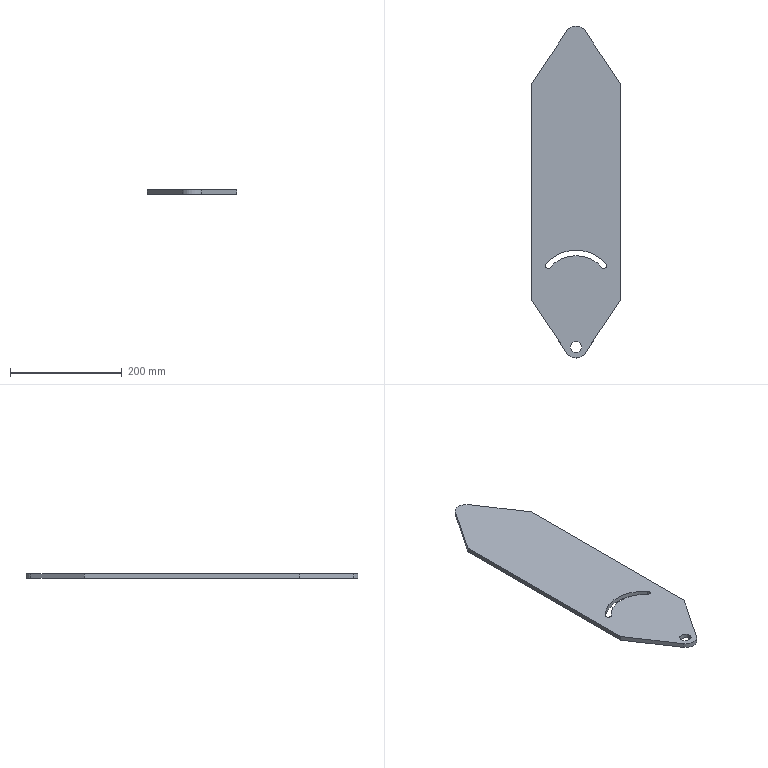Part | SolidWorks | features Cut 1, Extrusion 1 | 1 solid | 19 faces | box 160 x 594 x 8 mm | volume 632396 mm3 | plane 10 | cylinder 9 | commonest cylinder face diameters 10 x3 20 x2 40 x2 123.791 x1 143.791 x1
STEP:
#1=CARTESIAN_POINT('',(54.849,775.742,0.));
#2=VERTEX_POINT('',#1);
#3=CARTESIAN_POINT('',(53.575,779.077,0.));
#4=VERTEX_POINT('',#3);
#5=CARTESIAN_POINT('',(49.849,775.742,0.));
#6=DIRECTION('',(0.,0.,1.));
#7=DIRECTION('',(1.,0.,0.));
#8=AXIS2_PLACEMENT_3D('',#5,#6,#7);
#9=CIRCLE('',#8,5.);
#10=EDGE_CURVE('',#2,#4,#9,.T.);
#11=ORIENTED_EDGE('',*,*,#10,.F.);
#12=CARTESIAN_POINT('',(54.849,775.742,8.));
#13=VERTEX_POINT('',#12);
#14=CARTESIAN_POINT('',(54.849,775.742,-2.));
#15=DIRECTION('',(0.,0.,1.));
#16=VECTOR('',#15,1000.);
#17=LINE('',#14,#16);
#18=EDGE_CURVE('',#2,#13,#17,.T.);
#19=ORIENTED_EDGE('',*,*,#18,.T.);
#20=CARTESIAN_POINT('',(53.575,779.077,8.));
#21=VERTEX_POINT('',#20);
#22=CARTESIAN_POINT('',(49.849,775.742,8.));
#23=DIRECTION('',(0.,0.,1.));
#24=DIRECTION('',(1.,0.,0.));
#25=AXIS2_PLACEMENT_3D('',#22,#23,#24);
#26=CIRCLE('',#25,5.);
#27=EDGE_CURVE('',#13,#21,#26,.T.);
#28=ORIENTED_EDGE('',*,*,#27,.T.);
#29=CARTESIAN_POINT('',(53.575,779.077,-2.));
#30=DIRECTION('',(0.,0.,1.));
#31=VECTOR('',#30,1000.);
#32=LINE('',#29,#31);
#33=EDGE_CURVE('',#4,#21,#32,.T.);
#34=ORIENTED_EDGE('',*,*,#33,.F.);
#35=EDGE_LOOP('',(#11,#19,#28,#34));
#36=FACE_OUTER_BOUND('',#35,.T.);
#37=CARTESIAN_POINT('',(49.849,775.742,-2.));
#38=DIRECTION('',(0.,0.,1.));
#39=DIRECTION('',(1.,0.,0.));
#40=AXIS2_PLACEMENT_3D('',#37,#38,#39);
#41=CYLINDRICAL_SURFACE('',#40,5.);
#42=ADVANCED_FACE('',(#36),#41,.F.);
#43=CARTESIAN_POINT('',(-10.,630.,8.));
#44=VERTEX_POINT('',#43);
#45=CARTESIAN_POINT('',(10.,630.,8.));
#46=VERTEX_POINT('',#45);
#47=CARTESIAN_POINT('',(0.,630.,8.));
#48=DIRECTION('',(0.,0.,1.));
#49=DIRECTION('',(1.,0.,0.));
#50=AXIS2_PLACEMENT_3D('',#47,#48,#49);
#51=CIRCLE('',#50,10.);
#52=EDGE_CURVE('',#44,#46,#51,.T.);
#53=ORIENTED_EDGE('',*,*,#52,.T.);
#54=CARTESIAN_POINT('',(10.,630.,0.));
#55=VERTEX_POINT('',#54);
#56=CARTESIAN_POINT('',(10.,630.,8.));
#57=DIRECTION('',(0.,0.,-1.));
#58=VECTOR('',#57,1000.);
#59=LINE('',#56,#58);
#60=EDGE_CURVE('',#46,#55,#59,.T.);
#61=ORIENTED_EDGE('',*,*,#60,.T.);
#62=CARTESIAN_POINT('',(-10.,630.,0.));
#63=VERTEX_POINT('',#62);
#64=CARTESIAN_POINT('',(0.,630.,0.));
#65=DIRECTION('',(0.,0.,1.));
#66=DIRECTION('',(1.,0.,0.));
#67=AXIS2_PLACEMENT_3D('',#64,#65,#66);
#68=CIRCLE('',#67,10.);
#69=EDGE_CURVE('',#63,#55,#68,.T.);
#70=ORIENTED_EDGE('',*,*,#69,.F.);
#71=CARTESIAN_POINT('',(-10.,630.,8.));
#72=DIRECTION('',(0.,0.,-1.));
#73=VECTOR('',#72,1000.);
#74=LINE('',#71,#73);
#75=EDGE_CURVE('',#44,#63,#74,.T.);
#76=ORIENTED_EDGE('',*,*,#75,.F.);
#77=EDGE_LOOP('',(#53,#61,#70,#76));
#78=FACE_OUTER_BOUND('',#77,.T.);
#79=CARTESIAN_POINT('',(0.,630.,8.));
#80=DIRECTION('',(0.,0.,-1.));
#81=DIRECTION('',(-1.,0.,0.));
#82=AXIS2_PLACEMENT_3D('',#79,#80,#81);
#83=CYLINDRICAL_SURFACE('',#82,10.);
#84=ADVANCED_FACE('',(#78),#83,.F.);
#85=CARTESIAN_POINT('',(49.849,770.742,8.));
#86=VERTEX_POINT('',#85);
#87=CARTESIAN_POINT('',(49.849,775.742,8.));
#88=DIRECTION('',(0.,0.,1.));
#89=DIRECTION('',(1.,0.,0.));
#90=AXIS2_PLACEMENT_3D('',#87,#88,#89);
#91=CIRCLE('',#90,5.);
#92=EDGE_CURVE('',#86,#13,#91,.T.);
#93=ORIENTED_EDGE('',*,*,#92,.F.);
#94=CARTESIAN_POINT('',(47.561,770.742,8.));
#95=VERTEX_POINT('',#94);
#96=CARTESIAN_POINT('',(47.561,770.742,8.));
#97=DIRECTION('',(1.,0.,0.));
#98=VECTOR('',#97,1000.);
#99=LINE('',#96,#98);
#100=EDGE_CURVE('',#95,#86,#99,.T.);
#101=ORIENTED_EDGE('',*,*,#100,.F.);
#102=CARTESIAN_POINT('',(-47.561,770.742,8.));
#103=VERTEX_POINT('',#102);
#104=CARTESIAN_POINT('',(0.,731.132,8.));
#105=DIRECTION('',(0.,0.,-1.));
#106=DIRECTION('',(-1.,0.,0.));
#107=AXIS2_PLACEMENT_3D('',#104,#105,#106);
#108=CIRCLE('',#107,61.895);
#109=EDGE_CURVE('',#103,#95,#108,.T.);
#110=ORIENTED_EDGE('',*,*,#109,.F.);
#111=CARTESIAN_POINT('',(-49.849,770.742,8.));
#112=VERTEX_POINT('',#111);
#113=CARTESIAN_POINT('',(-49.849,770.742,8.));
#114=DIRECTION('',(1.,0.,0.));
#115=VECTOR('',#114,1000.);
#116=LINE('',#113,#115);
#117=EDGE_CURVE('',#112,#103,#116,.T.);
#118=ORIENTED_EDGE('',*,*,#117,.F.);
#119=CARTESIAN_POINT('',(-53.575,779.077,8.));
#120=VERTEX_POINT('',#119);
#121=CARTESIAN_POINT('',(-49.849,775.742,8.));
#122=DIRECTION('',(0.,0.,1.));
#123=DIRECTION('',(-1.,0.,0.));
#124=AXIS2_PLACEMENT_3D('',#121,#122,#123);
#125=CIRCLE('',#124,5.);
#126=EDGE_CURVE('',#120,#112,#125,.T.);
#127=ORIENTED_EDGE('',*,*,#126,.F.);
#128=CARTESIAN_POINT('',(0.,731.132,8.));
#129=DIRECTION('',(0.,0.,1.));
#130=DIRECTION('',(-1.,0.,0.));
#131=AXIS2_PLACEMENT_3D('',#128,#129,#130);
#132=CIRCLE('',#131,71.895);
#133=EDGE_CURVE('',#21,#120,#132,.T.);
#134=ORIENTED_EDGE('',*,*,#133,.F.);
#135=ORIENTED_EDGE('',*,*,#27,.F.);
#136=EDGE_LOOP('',(#93,#101,#110,#118,#127,#134,#135));
#137=FACE_BOUND('',#136,.T.);
#138=CARTESIAN_POINT('',(-16.639,1195.097,8.));
#139=VERTEX_POINT('',#138);
#140=CARTESIAN_POINT('',(-80.,1100.091,8.));
#141=VERTEX_POINT('',#140);
#142=CARTESIAN_POINT('',(-80.,1100.091,8.));
#143=DIRECTION('',(-0.5548,-0.832,0.));
#144=VECTOR('',#143,1000.);
#145=LINE('',#142,#144);
#146=EDGE_CURVE('',#139,#141,#145,.T.);
#147=ORIENTED_EDGE('',*,*,#146,.T.);
#148=CARTESIAN_POINT('',(-80.,713.909,8.));
#149=VERTEX_POINT('',#148);
#150=CARTESIAN_POINT('',(-80.,713.909,8.));
#151=DIRECTION('',(0.,-1.,0.));
#152=VECTOR('',#151,1000.);
#153=LINE('',#150,#152);
#154=EDGE_CURVE('',#141,#149,#153,.T.);
#155=ORIENTED_EDGE('',*,*,#154,.T.);
#156=CARTESIAN_POINT('',(-16.639,618.903,8.));
#157=VERTEX_POINT('',#156);
#158=CARTESIAN_POINT('',(-16.639,618.903,8.));
#159=DIRECTION('',(0.5548,-0.832,0.));
#160=VECTOR('',#159,1000.);
#161=LINE('',#158,#160);
#162=EDGE_CURVE('',#149,#157,#161,.T.);
#163=ORIENTED_EDGE('',*,*,#162,.T.);
#164=CARTESIAN_POINT('',(16.639,618.903,8.));
#165=VERTEX_POINT('',#164);
#166=CARTESIAN_POINT('',(0.,630.,8.));
#167=DIRECTION('',(0.,0.,1.));
#168=DIRECTION('',(1.,0.,0.));
#169=AXIS2_PLACEMENT_3D('',#166,#167,#168);
#170=CIRCLE('',#169,20.);
#171=EDGE_CURVE('',#157,#165,#170,.T.);
#172=ORIENTED_EDGE('',*,*,#171,.T.);
#173=CARTESIAN_POINT('',(80.,713.909,8.));
#174=VERTEX_POINT('',#173);
#175=CARTESIAN_POINT('',(16.639,618.903,8.));
#176=DIRECTION('',(0.5548,0.832,0.));
#177=VECTOR('',#176,1000.);
#178=LINE('',#175,#177);
#179=EDGE_CURVE('',#165,#174,#178,.T.);
#180=ORIENTED_EDGE('',*,*,#179,.T.);
#181=CARTESIAN_POINT('',(80.,1100.091,8.));
#182=VERTEX_POINT('',#181);
#183=CARTESIAN_POINT('',(80.,713.909,8.));
#184=DIRECTION('',(0.,1.,0.));
#185=VECTOR('',#184,1000.);
#186=LINE('',#183,#185);
#187=EDGE_CURVE('',#174,#182,#186,.T.);
#188=ORIENTED_EDGE('',*,*,#187,.T.);
#189=CARTESIAN_POINT('',(16.639,1195.097,8.));
#190=VERTEX_POINT('',#189);
#191=CARTESIAN_POINT('',(80.,1100.091,8.));
#192=DIRECTION('',(-0.5548,0.832,0.));
#193=VECTOR('',#192,1000.);
#194=LINE('',#191,#193);
#195=EDGE_CURVE('',#182,#190,#194,.T.);
#196=ORIENTED_EDGE('',*,*,#195,.T.);
#197=CARTESIAN_POINT('',(0.,1184.,8.));
#198=DIRECTION('',(0.,0.,1.));
#199=DIRECTION('',(1.,0.,0.));
#200=AXIS2_PLACEMENT_3D('',#197,#198,#199);
#201=CIRCLE('',#200,20.);
#202=EDGE_CURVE('',#190,#139,#201,.T.);
#203=ORIENTED_EDGE('',*,*,#202,.T.);
#204=EDGE_LOOP('',(#147,#155,#163,#172,#180,#188,#196,#203));
#205=FACE_OUTER_BOUND('',#204,.T.);
#206=ORIENTED_EDGE('',*,*,#52,.F.);
#207=CARTESIAN_POINT('',(0.,630.,8.));
#208=DIRECTION('',(0.,0.,1.));
#209=DIRECTION('',(1.,0.,0.));
#210=AXIS2_PLACEMENT_3D('',#207,#208,#209);
#211=CIRCLE('',#210,10.);
#212=EDGE_CURVE('',#46,#44,#211,.T.);
#213=ORIENTED_EDGE('',*,*,#212,.F.);
#214=EDGE_LOOP('',(#206,#213));
#215=FACE_BOUND('',#214,.T.);
#216=CARTESIAN_POINT('',(0.,1184.,8.));
#217=DIRECTION('',(0.,0.,1.));
#218=DIRECTION('',(1.,0.,0.));
#219=AXIS2_PLACEMENT_3D('',#216,#217,#218);
#220=PLANE('',#219);
#221=ADVANCED_FACE('',(#137,#205,#215),#220,.T.);
#222=CARTESIAN_POINT('',(47.561,770.742,0.));
#223=VERTEX_POINT('',#222);
#224=CARTESIAN_POINT('',(49.849,770.742,0.));
#225=VERTEX_POINT('',#224);
#226=CARTESIAN_POINT('',(0.,770.742,0.));
#227=DIRECTION('',(1.,0.,0.));
#228=VECTOR('',#227,1000.);
#229=LINE('',#226,#228);
#230=EDGE_CURVE('',#223,#225,#229,.T.);
#231=ORIENTED_EDGE('',*,*,#230,.T.);
#232=CARTESIAN_POINT('',(49.849,775.742,0.));
#233=DIRECTION('',(0.,0.,1.));
#234=DIRECTION('',(1.,0.,0.));
#235=AXIS2_PLACEMENT_3D('',#232,#233,#234);
#236=CIRCLE('',#235,5.);
#237=EDGE_CURVE('',#225,#2,#236,.T.);
#238=ORIENTED_EDGE('',*,*,#237,.T.);
#239=ORIENTED_EDGE('',*,*,#10,.T.);
#240=CARTESIAN_POINT('',(-53.575,779.077,0.));
#241=VERTEX_POINT('',#240);
#242=CARTESIAN_POINT('',(0.,731.132,0.));
#243=DIRECTION('',(0.,0.,1.));
#244=DIRECTION('',(1.,0.,0.));
#245=AXIS2_PLACEMENT_3D('',#242,#243,#244);
#246=CIRCLE('',#245,71.895);
#247=EDGE_CURVE('',#4,#241,#246,.T.);
#248=ORIENTED_EDGE('',*,*,#247,.T.);
#249=CARTESIAN_POINT('',(-49.849,770.742,0.));
#250=VERTEX_POINT('',#249);
#251=CARTESIAN_POINT('',(-49.849,775.742,0.));
#252=DIRECTION('',(0.,0.,1.));
#253=DIRECTION('',(1.,0.,0.));
#254=AXIS2_PLACEMENT_3D('',#251,#252,#253);
#255=CIRCLE('',#254,5.);
#256=EDGE_CURVE('',#241,#250,#255,.T.);
#257=ORIENTED_EDGE('',*,*,#256,.T.);
#258=CARTESIAN_POINT('',(-47.561,770.742,0.));
#259=VERTEX_POINT('',#258);
#260=CARTESIAN_POINT('',(0.,770.742,0.));
#261=DIRECTION('',(1.,0.,0.));
#262=VECTOR('',#261,1000.);
#263=LINE('',#260,#262);
#264=EDGE_CURVE('',#250,#259,#263,.T.);
#265=ORIENTED_EDGE('',*,*,#264,.T.);
#266=CARTESIAN_POINT('',(0.,731.132,0.));
#267=DIRECTION('',(0.,0.,-1.));
#268=DIRECTION('',(1.,0.,0.));
#269=AXIS2_PLACEMENT_3D('',#266,#267,#268);
#270=CIRCLE('',#269,61.895);
#271=EDGE_CURVE('',#259,#223,#270,.T.);
#272=ORIENTED_EDGE('',*,*,#271,.T.);
#273=EDGE_LOOP('',(#231,#238,#239,#248,#257,#265,#272));
#274=FACE_BOUND('',#273,.T.);
#275=CARTESIAN_POINT('',(-16.639,1195.097,0.));
#276=VERTEX_POINT('',#275);
#277=CARTESIAN_POINT('',(-80.,1100.091,0.));
#278=VERTEX_POINT('',#277);
#279=CARTESIAN_POINT('',(-80.,1100.091,0.));
#280=DIRECTION('',(-0.5548,-0.832,0.));
#281=VECTOR('',#280,1000.);
#282=LINE('',#279,#281);
#283=EDGE_CURVE('',#276,#278,#282,.T.);
#284=ORIENTED_EDGE('',*,*,#283,.F.);
#285=CARTESIAN_POINT('',(16.639,1195.097,0.));
#286=VERTEX_POINT('',#285);
#287=CARTESIAN_POINT('',(0.,1184.,0.));
#288=DIRECTION('',(0.,0.,1.));
#289=DIRECTION('',(1.,0.,0.));
#290=AXIS2_PLACEMENT_3D('',#287,#288,#289);
#291=CIRCLE('',#290,20.);
#292=EDGE_CURVE('',#286,#276,#291,.T.);
#293=ORIENTED_EDGE('',*,*,#292,.F.);
#294=CARTESIAN_POINT('',(80.,1100.091,0.));
#295=VERTEX_POINT('',#294);
#296=CARTESIAN_POINT('',(80.,1100.091,0.));
#297=DIRECTION('',(-0.5548,0.832,0.));
#298=VECTOR('',#297,1000.);
#299=LINE('',#296,#298);
#300=EDGE_CURVE('',#295,#286,#299,.T.);
#301=ORIENTED_EDGE('',*,*,#300,.F.);
#302=CARTESIAN_POINT('',(80.,713.909,0.));
#303=VERTEX_POINT('',#302);
#304=CARTESIAN_POINT('',(80.,713.909,0.));
#305=DIRECTION('',(0.,1.,0.));
#306=VECTOR('',#305,1000.);
#307=LINE('',#304,#306);
#308=EDGE_CURVE('',#303,#295,#307,.T.);
#309=ORIENTED_EDGE('',*,*,#308,.F.);
#310=CARTESIAN_POINT('',(16.639,618.903,0.));
#311=VERTEX_POINT('',#310);
#312=CARTESIAN_POINT('',(16.639,618.903,0.));
#313=DIRECTION('',(0.5548,0.832,0.));
#314=VECTOR('',#313,1000.);
#315=LINE('',#312,#314);
#316=EDGE_CURVE('',#311,#303,#315,.T.);
#317=ORIENTED_EDGE('',*,*,#316,.F.);
#318=CARTESIAN_POINT('',(-16.639,618.903,0.));
#319=VERTEX_POINT('',#318);
#320=CARTESIAN_POINT('',(0.,630.,0.));
#321=DIRECTION('',(0.,0.,1.));
#322=DIRECTION('',(1.,0.,0.));
#323=AXIS2_PLACEMENT_3D('',#320,#321,#322);
#324=CIRCLE('',#323,20.);
#325=EDGE_CURVE('',#319,#311,#324,.T.);
#326=ORIENTED_EDGE('',*,*,#325,.F.);
#327=CARTESIAN_POINT('',(-80.,713.909,0.));
#328=VERTEX_POINT('',#327);
#329=CARTESIAN_POINT('',(-16.639,618.903,0.));
#330=DIRECTION('',(0.5548,-0.832,0.));
#331=VECTOR('',#330,1000.);
#332=LINE('',#329,#331);
#333=EDGE_CURVE('',#328,#319,#332,.T.);
#334=ORIENTED_EDGE('',*,*,#333,.F.);
#335=CARTESIAN_POINT('',(-80.,713.909,0.));
#336=DIRECTION('',(0.,-1.,0.));
#337=VECTOR('',#336,1000.);
#338=LINE('',#335,#337);
#339=EDGE_CURVE('',#278,#328,#338,.T.);
#340=ORIENTED_EDGE('',*,*,#339,.F.);
#341=EDGE_LOOP('',(#284,#293,#301,#309,#317,#326,#334,#340));
#342=FACE_OUTER_BOUND('',#341,.T.);
#343=ORIENTED_EDGE('',*,*,#69,.T.);
#344=CARTESIAN_POINT('',(0.,630.,0.));
#345=DIRECTION('',(0.,0.,1.));
#346=DIRECTION('',(1.,0.,0.));
#347=AXIS2_PLACEMENT_3D('',#344,#345,#346);
#348=CIRCLE('',#347,10.);
#349=EDGE_CURVE('',#55,#63,#348,.T.);
#350=ORIENTED_EDGE('',*,*,#349,.T.);
#351=EDGE_LOOP('',(#343,#350));
#352=FACE_BOUND('',#351,.T.);
#353=CARTESIAN_POINT('',(0.,1184.,0.));
#354=DIRECTION('',(0.,0.,1.));
#355=DIRECTION('',(1.,0.,0.));
#356=AXIS2_PLACEMENT_3D('',#353,#354,#355);
#357=PLANE('',#356);
#358=ADVANCED_FACE('',(#274,#342,#352),#357,.F.);
#359=ORIENTED_EDGE('',*,*,#283,.T.);
#360=CARTESIAN_POINT('',(-80.,1100.091,8.));
#361=DIRECTION('',(0.,0.,-1.));
#362=VECTOR('',#361,1000.);
#363=LINE('',#360,#362);
#364=EDGE_CURVE('',#141,#278,#363,.T.);
#365=ORIENTED_EDGE('',*,*,#364,.F.);
#366=ORIENTED_EDGE('',*,*,#146,.F.);
#367=CARTESIAN_POINT('',(-16.639,1195.097,8.));
#368=DIRECTION('',(0.,0.,-1.));
#369=VECTOR('',#368,1000.);
#370=LINE('',#367,#369);
#371=EDGE_CURVE('',#139,#276,#370,.T.);
#372=ORIENTED_EDGE('',*,*,#371,.T.);
#373=EDGE_LOOP('',(#359,#365,#366,#372));
#374=FACE_OUTER_BOUND('',#373,.T.);
#375=CARTESIAN_POINT('',(-80.,1100.091,8.));
#376=DIRECTION('',(0.832,-0.5548,0.));
#377=DIRECTION('',(0.5548,0.832,0.));
#378=AXIS2_PLACEMENT_3D('',#375,#376,#377);
#379=PLANE('',#378);
#380=ADVANCED_FACE('',(#374),#379,.F.);
#381=ORIENTED_EDGE('',*,*,#339,.T.);
#382=CARTESIAN_POINT('',(-80.,713.909,8.));
#383=DIRECTION('',(0.,0.,-1.));
#384=VECTOR('',#383,1000.);
#385=LINE('',#382,#384);
#386=EDGE_CURVE('',#149,#328,#385,.T.);
#387=ORIENTED_EDGE('',*,*,#386,.F.);
#388=ORIENTED_EDGE('',*,*,#154,.F.);
#389=ORIENTED_EDGE('',*,*,#364,.T.);
#390=EDGE_LOOP('',(#381,#387,#388,#389));
#391=FACE_OUTER_BOUND('',#390,.T.);
#392=CARTESIAN_POINT('',(-80.,713.909,8.));
#393=DIRECTION('',(1.,0.,0.));
#394=DIRECTION('',(0.,0.,-1.));
#395=AXIS2_PLACEMENT_3D('',#392,#393,#394);
#396=PLANE('',#395);
#397=ADVANCED_FACE('',(#391),#396,.F.);
#398=ORIENTED_EDGE('',*,*,#333,.T.);
#399=CARTESIAN_POINT('',(-16.639,618.903,8.));
#400=DIRECTION('',(0.,0.,-1.));
#401=VECTOR('',#400,1000.);
#402=LINE('',#399,#401);
#403=EDGE_CURVE('',#157,#319,#402,.T.);
#404=ORIENTED_EDGE('',*,*,#403,.F.);
#405=ORIENTED_EDGE('',*,*,#162,.F.);
#406=ORIENTED_EDGE('',*,*,#386,.T.);
#407=EDGE_LOOP('',(#398,#404,#405,#406));
#408=FACE_OUTER_BOUND('',#407,.T.);
#409=CARTESIAN_POINT('',(-16.639,618.903,8.));
#410=DIRECTION('',(0.832,0.5548,0.));
#411=DIRECTION('',(-0.5548,0.832,0.));
#412=AXIS2_PLACEMENT_3D('',#409,#410,#411);
#413=PLANE('',#412);
#414=ADVANCED_FACE('',(#408),#413,.F.);
#415=ORIENTED_EDGE('',*,*,#325,.T.);
#416=CARTESIAN_POINT('',(16.639,618.903,8.));
#417=DIRECTION('',(0.,0.,-1.));
#418=VECTOR('',#417,1000.);
#419=LINE('',#416,#418);
#420=EDGE_CURVE('',#165,#311,#419,.T.);
#421=ORIENTED_EDGE('',*,*,#420,.F.);
#422=ORIENTED_EDGE('',*,*,#171,.F.);
#423=ORIENTED_EDGE('',*,*,#403,.T.);
#424=EDGE_LOOP('',(#415,#421,#422,#423));
#425=FACE_OUTER_BOUND('',#424,.T.);
#426=CARTESIAN_POINT('',(0.,630.,8.));
#427=DIRECTION('',(0.,0.,-1.));
#428=DIRECTION('',(-1.,0.,0.));
#429=AXIS2_PLACEMENT_3D('',#426,#427,#428);
#430=CYLINDRICAL_SURFACE('',#429,20.);
#431=ADVANCED_FACE('',(#425),#430,.T.);
#432=ORIENTED_EDGE('',*,*,#316,.T.);
#433=CARTESIAN_POINT('',(80.,713.909,8.));
#434=DIRECTION('',(0.,0.,-1.));
#435=VECTOR('',#434,1000.);
#436=LINE('',#433,#435);
#437=EDGE_CURVE('',#174,#303,#436,.T.);
#438=ORIENTED_EDGE('',*,*,#437,.F.);
#439=ORIENTED_EDGE('',*,*,#179,.F.);
#440=ORIENTED_EDGE('',*,*,#420,.T.);
#441=EDGE_LOOP('',(#432,#438,#439,#440));
#442=FACE_OUTER_BOUND('',#441,.T.);
#443=CARTESIAN_POINT('',(16.639,618.903,8.));
#444=DIRECTION('',(-0.832,0.5548,0.));
#445=DIRECTION('',(-0.5548,-0.832,0.));
#446=AXIS2_PLACEMENT_3D('',#443,#444,#445);
#447=PLANE('',#446);
#448=ADVANCED_FACE('',(#442),#447,.F.);
#449=ORIENTED_EDGE('',*,*,#308,.T.);
#450=CARTESIAN_POINT('',(80.,1100.091,8.));
#451=DIRECTION('',(0.,0.,-1.));
#452=VECTOR('',#451,1000.);
#453=LINE('',#450,#452);
#454=EDGE_CURVE('',#182,#295,#453,.T.);
#455=ORIENTED_EDGE('',*,*,#454,.F.);
#456=ORIENTED_EDGE('',*,*,#187,.F.);
#457=ORIENTED_EDGE('',*,*,#437,.T.);
#458=EDGE_LOOP('',(#449,#455,#456,#457));
#459=FACE_OUTER_BOUND('',#458,.T.);
#460=CARTESIAN_POINT('',(80.,713.909,8.));
#461=DIRECTION('',(-1.,0.,0.));
#462=DIRECTION('',(0.,0.,1.));
#463=AXIS2_PLACEMENT_3D('',#460,#461,#462);
#464=PLANE('',#463);
#465=ADVANCED_FACE('',(#459),#464,.F.);
#466=ORIENTED_EDGE('',*,*,#300,.T.);
#467=CARTESIAN_POINT('',(16.639,1195.097,8.));
#468=DIRECTION('',(0.,0.,-1.));
#469=VECTOR('',#468,1000.);
#470=LINE('',#467,#469);
#471=EDGE_CURVE('',#190,#286,#470,.T.);
#472=ORIENTED_EDGE('',*,*,#471,.F.);
#473=ORIENTED_EDGE('',*,*,#195,.F.);
#474=ORIENTED_EDGE('',*,*,#454,.T.);
#475=EDGE_LOOP('',(#466,#472,#473,#474));
#476=FACE_OUTER_BOUND('',#475,.T.);
#477=CARTESIAN_POINT('',(80.,1100.091,8.));
#478=DIRECTION('',(-0.832,-0.5548,0.));
#479=DIRECTION('',(0.5548,-0.832,0.));
#480=AXIS2_PLACEMENT_3D('',#477,#478,#479);
#481=PLANE('',#480);
#482=ADVANCED_FACE('',(#476),#481,.F.);
#483=ORIENTED_EDGE('',*,*,#292,.T.);
#484=ORIENTED_EDGE('',*,*,#371,.F.);
#485=ORIENTED_EDGE('',*,*,#202,.F.);
#486=ORIENTED_EDGE('',*,*,#471,.T.);
#487=EDGE_LOOP('',(#483,#484,#485,#486));
#488=FACE_OUTER_BOUND('',#487,.T.);
#489=CARTESIAN_POINT('',(0.,1184.,8.));
#490=DIRECTION('',(0.,0.,-1.));
#491=DIRECTION('',(-1.,0.,0.));
#492=AXIS2_PLACEMENT_3D('',#489,#490,#491);
#493=CYLINDRICAL_SURFACE('',#492,20.);
#494=ADVANCED_FACE('',(#488),#493,.T.);
#495=ORIENTED_EDGE('',*,*,#60,.F.);
#496=ORIENTED_EDGE('',*,*,#212,.T.);
#497=ORIENTED_EDGE('',*,*,#75,.T.);
#498=ORIENTED_EDGE('',*,*,#349,.F.);
#499=EDGE_LOOP('',(#495,#496,#497,#498));
#500=FACE_OUTER_BOUND('',#499,.T.);
#501=CARTESIAN_POINT('',(0.,630.,8.));
#502=DIRECTION('',(0.,0.,-1.));
#503=DIRECTION('',(-1.,0.,0.));
#504=AXIS2_PLACEMENT_3D('',#501,#502,#503);
#505=CYLINDRICAL_SURFACE('',#504,10.);
#506=ADVANCED_FACE('',(#500),#505,.F.);
#507=ORIENTED_EDGE('',*,*,#18,.F.);
#508=ORIENTED_EDGE('',*,*,#237,.F.);
#509=CARTESIAN_POINT('',(49.849,770.742,-2.));
#510=DIRECTION('',(0.,0.,1.));
#511=VECTOR('',#510,1000.);
#512=LINE('',#509,#511);
#513=EDGE_CURVE('',#225,#86,#512,.T.);
#514=ORIENTED_EDGE('',*,*,#513,.T.);
#515=ORIENTED_EDGE('',*,*,#92,.T.);
#516=EDGE_LOOP('',(#507,#508,#514,#515));
#517=FACE_OUTER_BOUND('',#516,.T.);
#518=CARTESIAN_POINT('',(49.849,775.742,-2.));
#519=DIRECTION('',(0.,0.,1.));
#520=DIRECTION('',(1.,0.,0.));
#521=AXIS2_PLACEMENT_3D('',#518,#519,#520);
#522=CYLINDRICAL_SURFACE('',#521,5.);
#523=ADVANCED_FACE('',(#517),#522,.F.);
#524=CARTESIAN_POINT('',(47.561,770.742,-2.));
#525=DIRECTION('',(0.,0.,1.));
#526=VECTOR('',#525,1000.);
#527=LINE('',#524,#526);
#528=EDGE_CURVE('',#223,#95,#527,.T.);
#529=ORIENTED_EDGE('',*,*,#528,.T.);
#530=ORIENTED_EDGE('',*,*,#100,.T.);
#531=ORIENTED_EDGE('',*,*,#513,.F.);
#532=ORIENTED_EDGE('',*,*,#230,.F.);
#533=EDGE_LOOP('',(#529,#530,#531,#532));
#534=FACE_OUTER_BOUND('',#533,.T.);
#535=CARTESIAN_POINT('',(47.561,770.742,-2.));
#536=DIRECTION('',(0.,-1.,0.));
#537=DIRECTION('',(0.,0.,-1.));
#538=AXIS2_PLACEMENT_3D('',#535,#536,#537);
#539=PLANE('',#538);
#540=ADVANCED_FACE('',(#534),#539,.F.);
#541=CARTESIAN_POINT('',(-47.561,770.742,-2.));
#542=DIRECTION('',(0.,0.,1.));
#543=VECTOR('',#542,1000.);
#544=LINE('',#541,#543);
#545=EDGE_CURVE('',#259,#103,#544,.T.);
#546=ORIENTED_EDGE('',*,*,#545,.T.);
#547=ORIENTED_EDGE('',*,*,#109,.T.);
#548=ORIENTED_EDGE('',*,*,#528,.F.);
#549=ORIENTED_EDGE('',*,*,#271,.F.);
#550=EDGE_LOOP('',(#546,#547,#548,#549));
#551=FACE_OUTER_BOUND('',#550,.T.);
#552=CARTESIAN_POINT('',(0.,731.132,-2.));
#553=DIRECTION('',(0.,0.,1.));
#554=DIRECTION('',(1.,0.,0.));
#555=AXIS2_PLACEMENT_3D('',#552,#553,#554);
#556=CYLINDRICAL_SURFACE('',#555,61.895);
#557=ADVANCED_FACE('',(#551),#556,.T.);
#558=CARTESIAN_POINT('',(-49.849,770.742,-2.));
#559=DIRECTION('',(0.,0.,1.));
#560=VECTOR('',#559,1000.);
#561=LINE('',#558,#560);
#562=EDGE_CURVE('',#250,#112,#561,.T.);
#563=ORIENTED_EDGE('',*,*,#562,.T.);
#564=ORIENTED_EDGE('',*,*,#117,.T.);
#565=ORIENTED_EDGE('',*,*,#545,.F.);
#566=ORIENTED_EDGE('',*,*,#264,.F.);
#567=EDGE_LOOP('',(#563,#564,#565,#566));
#568=FACE_OUTER_BOUND('',#567,.T.);
#569=CARTESIAN_POINT('',(-49.849,770.742,-2.));
#570=DIRECTION('',(0.,-1.,0.));
#571=DIRECTION('',(0.,0.,-1.));
#572=AXIS2_PLACEMENT_3D('',#569,#570,#571);
#573=PLANE('',#572);
#574=ADVANCED_FACE('',(#568),#573,.F.);
#575=CARTESIAN_POINT('',(-53.575,779.077,-2.));
#576=DIRECTION('',(0.,0.,1.));
#577=VECTOR('',#576,1000.);
#578=LINE('',#575,#577);
#579=EDGE_CURVE('',#241,#120,#578,.T.);
#580=ORIENTED_EDGE('',*,*,#579,.T.);
#581=ORIENTED_EDGE('',*,*,#126,.T.);
#582=ORIENTED_EDGE('',*,*,#562,.F.);
#583=ORIENTED_EDGE('',*,*,#256,.F.);
#584=EDGE_LOOP('',(#580,#581,#582,#583));
#585=FACE_OUTER_BOUND('',#584,.T.);
#586=CARTESIAN_POINT('',(-49.849,775.742,-2.));
#587=DIRECTION('',(0.,0.,1.));
#588=DIRECTION('',(1.,0.,0.));
#589=AXIS2_PLACEMENT_3D('',#586,#587,#588);
#590=CYLINDRICAL_SURFACE('',#589,5.);
#591=ADVANCED_FACE('',(#585),#590,.F.);
#592=ORIENTED_EDGE('',*,*,#33,.T.);
#593=ORIENTED_EDGE('',*,*,#133,.T.);
#594=ORIENTED_EDGE('',*,*,#579,.F.);
#595=ORIENTED_EDGE('',*,*,#247,.F.);
#596=EDGE_LOOP('',(#592,#593,#594,#595));
#597=FACE_OUTER_BOUND('',#596,.T.);
#598=CARTESIAN_POINT('',(0.,731.132,-2.));
#599=DIRECTION('',(0.,0.,1.));
#600=DIRECTION('',(1.,0.,0.));
#601=AXIS2_PLACEMENT_3D('',#598,#599,#600);
#602=CYLINDRICAL_SURFACE('',#601,71.895);
#603=ADVANCED_FACE('',(#597),#602,.F.);
#604=CLOSED_SHELL('',(#42,#84,#221,#358,#380,#397,#414,#431,#448,#465,#482,#494,#506,#523,#540,#557,#574,#591,#603));
#605=MANIFOLD_SOLID_BREP('',#604);
#606=CARTESIAN_POINT('',(0.,0.,0.));
#607=DIRECTION('',(0.,0.,1.));
#608=DIRECTION('',(1.,0.,0.));
#609=AXIS2_PLACEMENT_3D('',#606,#607,#608);
#610=(LENGTH_UNIT()NAMED_UNIT(*)SI_UNIT(.MILLI.,.METRE.));
#611=UNCERTAINTY_MEASURE_WITH_UNIT(LENGTH_MEASURE(0.00001),#610,'','');
#612=(NAMED_UNIT(*)PLANE_ANGLE_UNIT()SI_UNIT($,.RADIAN.));
#613=(NAMED_UNIT(*)SI_UNIT($,.STERADIAN.)SOLID_ANGLE_UNIT());
#614=(GEOMETRIC_REPRESENTATION_CONTEXT(3)GLOBAL_UNCERTAINTY_ASSIGNED_CONTEXT((#611))GLOBAL_UNIT_ASSIGNED_CONTEXT((#610,#612,#613))REPRESENTATION_CONTEXT('',''));
#615=ADVANCED_BREP_SHAPE_REPRESENTATION('',(#605,#609),#614);